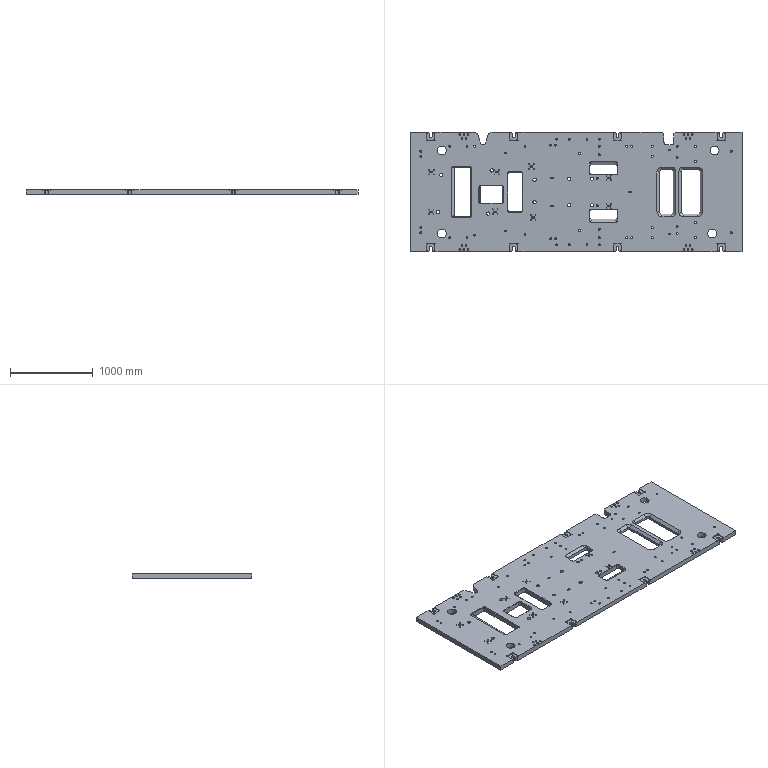Part | STEP file | lll_id4834_x_t | 1 solid | 601 faces | box 4000 x 1440 x 60 mm | volume 301601581 mm3 | cylinder 287 | plane 199 | cone 107 | spline 8 | commonest cylinder face diameters 23.009 x46 34.008 x46 40 x36 6.806 x32 8.506 x32 16 x22